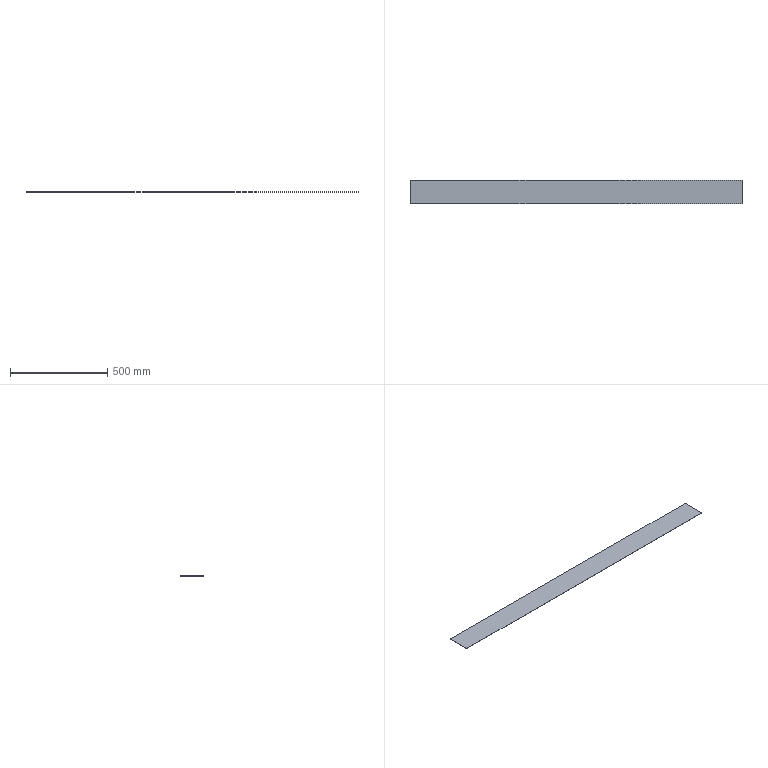Part | SolidWorks | features BaseBody 1 | 1 solid | 6 faces | box 1703 x 120 x 1 mm | volume 204360 mm3 | plane 6
STEP:
#1=CARTESIAN_POINT('',(-819.,70.,1.5));
#2=VERTEX_POINT('',#1);
#3=CARTESIAN_POINT('',(884.,70.,1.5));
#4=VERTEX_POINT('',#3);
#5=CARTESIAN_POINT('',(32.5,70.,1.5));
#6=DIRECTION('',(1.,0.,0.));
#7=VECTOR('',#6,1000.);
#8=LINE('',#5,#7);
#9=EDGE_CURVE('',#2,#4,#8,.T.);
#10=ORIENTED_EDGE('',*,*,#9,.T.);
#11=CARTESIAN_POINT('',(884.,-50.,1.5));
#12=VERTEX_POINT('',#11);
#13=CARTESIAN_POINT('',(884.,10.,1.5));
#14=DIRECTION('',(0.,-1.,0.));
#15=VECTOR('',#14,1000.);
#16=LINE('',#13,#15);
#17=EDGE_CURVE('',#4,#12,#16,.T.);
#18=ORIENTED_EDGE('',*,*,#17,.T.);
#19=CARTESIAN_POINT('',(-819.,-50.,1.5));
#20=VERTEX_POINT('',#19);
#21=CARTESIAN_POINT('',(32.5,-50.,1.5));
#22=DIRECTION('',(-1.,0.,0.));
#23=VECTOR('',#22,1000.);
#24=LINE('',#21,#23);
#25=EDGE_CURVE('',#12,#20,#24,.T.);
#26=ORIENTED_EDGE('',*,*,#25,.T.);
#27=CARTESIAN_POINT('',(-819.,10.,1.5));
#28=DIRECTION('',(0.,1.,0.));
#29=VECTOR('',#28,1000.);
#30=LINE('',#27,#29);
#31=EDGE_CURVE('',#20,#2,#30,.T.);
#32=ORIENTED_EDGE('',*,*,#31,.T.);
#33=EDGE_LOOP('',(#10,#18,#26,#32));
#34=FACE_OUTER_BOUND('',#33,.T.);
#35=CARTESIAN_POINT('',(32.5,10.,1.5));
#36=DIRECTION('',(0.,0.,-1.));
#37=DIRECTION('',(0.,1.,0.));
#38=AXIS2_PLACEMENT_3D('',#35,#36,#37);
#39=PLANE('',#38);
#40=ADVANCED_FACE('',(#34),#39,.T.);
#41=CARTESIAN_POINT('',(884.,70.,2.5));
#42=VERTEX_POINT('',#41);
#43=CARTESIAN_POINT('',(884.,-50.,2.5));
#44=VERTEX_POINT('',#43);
#45=CARTESIAN_POINT('',(884.,10.,2.5));
#46=DIRECTION('',(0.,-1.,0.));
#47=VECTOR('',#46,1000.);
#48=LINE('',#45,#47);
#49=EDGE_CURVE('',#42,#44,#48,.T.);
#50=ORIENTED_EDGE('',*,*,#49,.T.);
#51=CARTESIAN_POINT('',(884.,-50.,2.));
#52=DIRECTION('',(0.,0.,-1.));
#53=VECTOR('',#52,1000.);
#54=LINE('',#51,#53);
#55=EDGE_CURVE('',#44,#12,#54,.T.);
#56=ORIENTED_EDGE('',*,*,#55,.T.);
#57=ORIENTED_EDGE('',*,*,#17,.F.);
#58=CARTESIAN_POINT('',(884.,70.,2.));
#59=DIRECTION('',(0.,0.,1.));
#60=VECTOR('',#59,1000.);
#61=LINE('',#58,#60);
#62=EDGE_CURVE('',#4,#42,#61,.T.);
#63=ORIENTED_EDGE('',*,*,#62,.T.);
#64=EDGE_LOOP('',(#50,#56,#57,#63));
#65=FACE_OUTER_BOUND('',#64,.T.);
#66=CARTESIAN_POINT('',(884.,10.,2.));
#67=DIRECTION('',(1.,0.,0.));
#68=DIRECTION('',(0.,1.,0.));
#69=AXIS2_PLACEMENT_3D('',#66,#67,#68);
#70=PLANE('',#69);
#71=ADVANCED_FACE('',(#65),#70,.T.);
#72=CARTESIAN_POINT('',(-819.,70.,2.5));
#73=VERTEX_POINT('',#72);
#74=CARTESIAN_POINT('',(32.5,70.,2.5));
#75=DIRECTION('',(1.,0.,0.));
#76=VECTOR('',#75,1000.);
#77=LINE('',#74,#76);
#78=EDGE_CURVE('',#73,#42,#77,.T.);
#79=ORIENTED_EDGE('',*,*,#78,.T.);
#80=ORIENTED_EDGE('',*,*,#62,.F.);
#81=ORIENTED_EDGE('',*,*,#9,.F.);
#82=CARTESIAN_POINT('',(-819.,70.,2.));
#83=DIRECTION('',(0.,0.,1.));
#84=VECTOR('',#83,1000.);
#85=LINE('',#82,#84);
#86=EDGE_CURVE('',#2,#73,#85,.T.);
#87=ORIENTED_EDGE('',*,*,#86,.T.);
#88=EDGE_LOOP('',(#79,#80,#81,#87));
#89=FACE_OUTER_BOUND('',#88,.T.);
#90=CARTESIAN_POINT('',(32.5,70.,2.));
#91=DIRECTION('',(0.,1.,0.));
#92=DIRECTION('',(0.,0.,1.));
#93=AXIS2_PLACEMENT_3D('',#90,#91,#92);
#94=PLANE('',#93);
#95=ADVANCED_FACE('',(#89),#94,.T.);
#96=CARTESIAN_POINT('',(-819.,-50.,2.5));
#97=VERTEX_POINT('',#96);
#98=CARTESIAN_POINT('',(-819.,10.,2.5));
#99=DIRECTION('',(0.,1.,0.));
#100=VECTOR('',#99,1000.);
#101=LINE('',#98,#100);
#102=EDGE_CURVE('',#97,#73,#101,.T.);
#103=ORIENTED_EDGE('',*,*,#102,.T.);
#104=ORIENTED_EDGE('',*,*,#86,.F.);
#105=ORIENTED_EDGE('',*,*,#31,.F.);
#106=CARTESIAN_POINT('',(-819.,-50.,2.));
#107=DIRECTION('',(0.,0.,1.));
#108=VECTOR('',#107,1000.);
#109=LINE('',#106,#108);
#110=EDGE_CURVE('',#20,#97,#109,.T.);
#111=ORIENTED_EDGE('',*,*,#110,.T.);
#112=EDGE_LOOP('',(#103,#104,#105,#111));
#113=FACE_OUTER_BOUND('',#112,.T.);
#114=CARTESIAN_POINT('',(-819.,10.,2.));
#115=DIRECTION('',(-1.,0.,0.));
#116=DIRECTION('',(0.,0.,1.));
#117=AXIS2_PLACEMENT_3D('',#114,#115,#116);
#118=PLANE('',#117);
#119=ADVANCED_FACE('',(#113),#118,.T.);
#120=CARTESIAN_POINT('',(32.5,-50.,2.5));
#121=DIRECTION('',(-1.,0.,0.));
#122=VECTOR('',#121,1000.);
#123=LINE('',#120,#122);
#124=EDGE_CURVE('',#44,#97,#123,.T.);
#125=ORIENTED_EDGE('',*,*,#124,.T.);
#126=ORIENTED_EDGE('',*,*,#110,.F.);
#127=ORIENTED_EDGE('',*,*,#25,.F.);
#128=ORIENTED_EDGE('',*,*,#55,.F.);
#129=EDGE_LOOP('',(#125,#126,#127,#128));
#130=FACE_OUTER_BOUND('',#129,.T.);
#131=CARTESIAN_POINT('',(32.5,-50.,2.));
#132=DIRECTION('',(0.,-1.,0.));
#133=DIRECTION('',(0.,0.,-1.));
#134=AXIS2_PLACEMENT_3D('',#131,#132,#133);
#135=PLANE('',#134);
#136=ADVANCED_FACE('',(#130),#135,.T.);
#137=ORIENTED_EDGE('',*,*,#78,.F.);
#138=ORIENTED_EDGE('',*,*,#102,.F.);
#139=ORIENTED_EDGE('',*,*,#124,.F.);
#140=ORIENTED_EDGE('',*,*,#49,.F.);
#141=EDGE_LOOP('',(#137,#138,#139,#140));
#142=FACE_OUTER_BOUND('',#141,.T.);
#143=CARTESIAN_POINT('',(32.5,10.,2.5));
#144=DIRECTION('',(0.,0.,1.));
#145=DIRECTION('',(0.,-1.,0.));
#146=AXIS2_PLACEMENT_3D('',#143,#144,#145);
#147=PLANE('',#146);
#148=ADVANCED_FACE('',(#142),#147,.T.);
#149=CLOSED_SHELL('',(#40,#71,#95,#119,#136,#148));
#150=MANIFOLD_SOLID_BREP('',#149);
#151=CARTESIAN_POINT('',(0.,0.,0.));
#152=DIRECTION('',(0.,0.,1.));
#153=DIRECTION('',(1.,0.,0.));
#154=AXIS2_PLACEMENT_3D('',#151,#152,#153);
#155=(LENGTH_UNIT()NAMED_UNIT(*)SI_UNIT(.MILLI.,.METRE.));
#156=UNCERTAINTY_MEASURE_WITH_UNIT(LENGTH_MEASURE(0.00001),#155,'','');
#157=(NAMED_UNIT(*)PLANE_ANGLE_UNIT()SI_UNIT($,.RADIAN.));
#158=(NAMED_UNIT(*)SI_UNIT($,.STERADIAN.)SOLID_ANGLE_UNIT());
#159=(GEOMETRIC_REPRESENTATION_CONTEXT(3)GLOBAL_UNCERTAINTY_ASSIGNED_CONTEXT((#156))GLOBAL_UNIT_ASSIGNED_CONTEXT((#155,#157,#158))REPRESENTATION_CONTEXT('',''));
#160=ADVANCED_BREP_SHAPE_REPRESENTATION('',(#150,#154),#159);